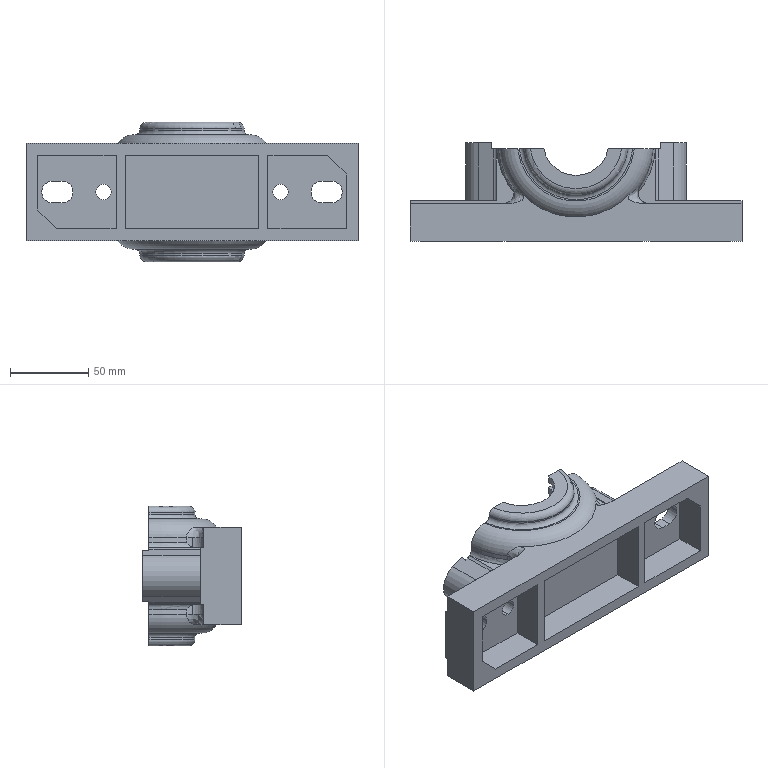Part | SolidWorks | features ICE 6, MirrorPattern 2, VarFillet 2, CombineBodies 1, MoveCopyBody 1, RevCut 1, Revolution 1, Stock 1 | 1 solid | 111 faces | box 212 x 63 x 89 mm | volume 296687 mm3 | plane 54 | cylinder 39 | torus 12 | spline 4 | cone 2 | commonest cylinder face diameters 14 x10 10 x8 42 x4 99 x4 113 x4 28 x2